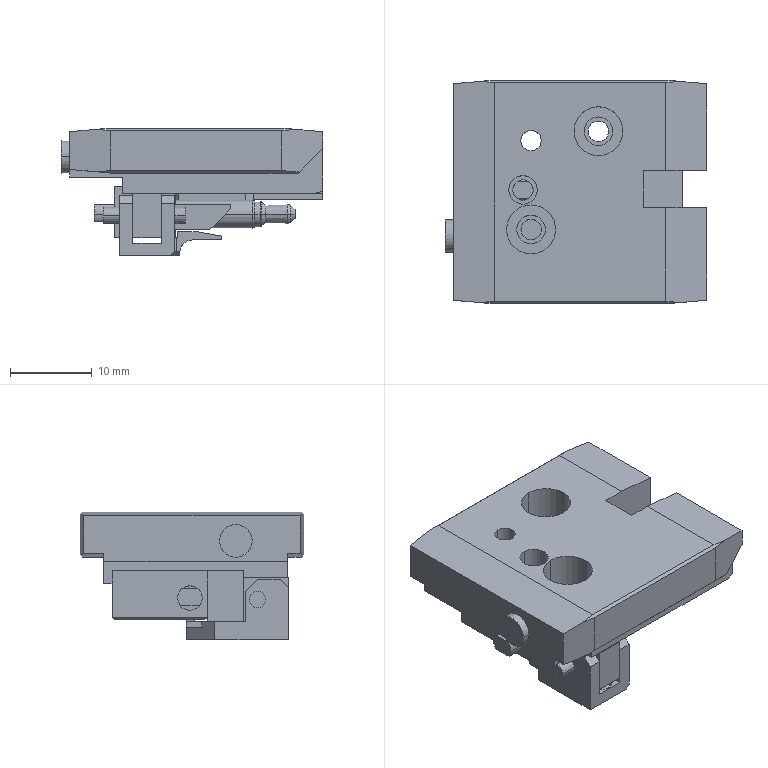Part | NX | 8 solids | 205 faces | box 32 x 27.4 x 15.65 mm | volume 6582 mm3 | plane 136 | cylinder 52 | cone 9 | torus 8 | commonest cylinder face diameters 2 x8 2.5 x8 3.5 x8 3.1 x6 6 x6 3 x5